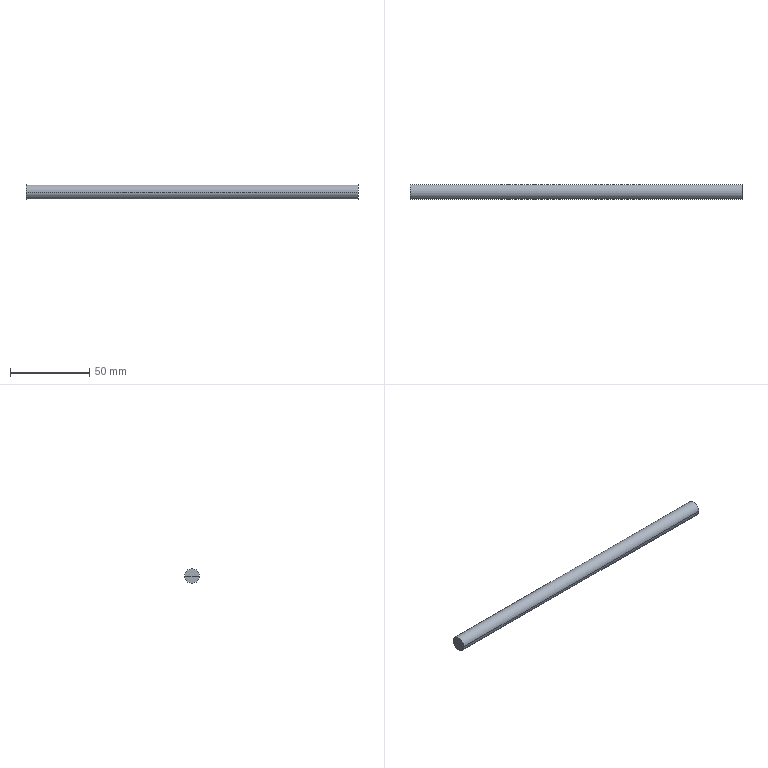Part | STEP file | BREP_8 | 1 solid | 6 faces | box 210 x 9.4 x 9.4 mm | volume 14574 mm3 | plane 4 | cylinder 2 | commonest cylinder face diameters 9.4 x2
STEP:
#1=CARTESIAN_POINT('',(0.,0.,0.));
#2=DIRECTION('',(0.,0.,1.));
#3=DIRECTION('',(1.,0.,0.));
#4=AXIS2_PLACEMENT_3D('',#1,#2,#3);
#5=CARTESIAN_POINT('',(-105.,0.,0.));
#6=VERTEX_POINT('',#5);
#7=CARTESIAN_POINT('',(-105.,-4.7,0.));
#8=VERTEX_POINT('',#7);
#9=CARTESIAN_POINT('',(-105.,0.,0.));
#10=DIRECTION('',(0.,-1.,0.));
#11=VECTOR('',#10,1.);
#12=LINE('',#9,#11);
#13=CARTESIAN_POINT('',(-105.,0.,-2.35));
#14=DIRECTION('',(1.,0.,0.));
#15=DIRECTION('',(0.,-1.,0.));
#16=AXIS2_PLACEMENT_3D('',#13,#14,#15);
#17=PLANE('',#16);
#18=CARTESIAN_POINT('',(0.,-2.35));
#19=DIRECTION('',(1.,0.));
#20=VECTOR('',#19,1.);
#21=LINE('',#18,#20);
#22=(GEOMETRIC_REPRESENTATION_CONTEXT(2)PARAMETRIC_REPRESENTATION_CONTEXT()REPRESENTATION_CONTEXT('',''));
#23=DEFINITIONAL_REPRESENTATION('',(#21),#22);
#24=PCURVE('',#17,#23);
#25=CARTESIAN_POINT('',(-105.,0.,2.35));
#26=DIRECTION('',(1.,0.,0.));
#27=DIRECTION('',(0.,1.,0.));
#28=AXIS2_PLACEMENT_3D('',#25,#26,#27);
#29=PLANE('',#28);
#30=CARTESIAN_POINT('',(0.,-2.35));
#31=DIRECTION('',(-1.,0.));
#32=VECTOR('',#31,1.);
#33=LINE('',#30,#32);
#34=(GEOMETRIC_REPRESENTATION_CONTEXT(2)PARAMETRIC_REPRESENTATION_CONTEXT()REPRESENTATION_CONTEXT('',''));
#35=DEFINITIONAL_REPRESENTATION('',(#33),#34);
#36=PCURVE('',#29,#35);
#37=SURFACE_CURVE('',#12,(#24,#36),.PCURVE_S1.);
#38=EDGE_CURVE('',#6,#8,#37,.T.);
#39=ORIENTED_EDGE('',*,*,#38,.T.);
#40=CARTESIAN_POINT('',(-105.,4.7,0.));
#41=VERTEX_POINT('',#40);
#42=CARTESIAN_POINT('',(-105.,0.,0.));
#43=DIRECTION('',(-1.,0.,0.));
#44=DIRECTION('',(0.,1.,0.));
#45=AXIS2_PLACEMENT_3D('',#42,#43,#44);
#46=CIRCLE('',#45,4.7);
#47=CARTESIAN_POINT('',(-4.7,-2.35));
#48=CARTESIAN_POINT('',(-4.7,5.791));
#49=CARTESIAN_POINT('',(2.35,1.72));
#50=CARTESIAN_POINT('',(9.4,-2.35));
#51=CARTESIAN_POINT('',(2.35,-6.42));
#52=CARTESIAN_POINT('',(-4.7,-10.491));
#53=CARTESIAN_POINT('',(-4.7,-2.35));
#54=(BOUNDED_CURVE()B_SPLINE_CURVE(2,(#47,#48,#49,#50,#51,#52,#53),.UNSPECIFIED.,.T.,.F.)B_SPLINE_CURVE_WITH_KNOTS((1,2,2,2,2,1),(-2.094,0.,2.094,4.189,6.283,8.378),.UNSPECIFIED.)CURVE()GEOMETRIC_REPRESENTATION_ITEM()RATIONAL_B_SPLINE_CURVE((1.,0.5,1.,0.5,1.,0.5,1.))REPRESENTATION_ITEM(''));
#55=(GEOMETRIC_REPRESENTATION_CONTEXT(2)PARAMETRIC_REPRESENTATION_CONTEXT()REPRESENTATION_CONTEXT('',''));
#56=DEFINITIONAL_REPRESENTATION('',(#54),#55);
#57=PCURVE('',#17,#56);
#58=CARTESIAN_POINT('',(0.,0.,0.));
#59=DIRECTION('',(-1.,0.,0.));
#60=DIRECTION('',(0.,1.,0.));
#61=AXIS2_PLACEMENT_3D('',#58,#59,#60);
#62=CYLINDRICAL_SURFACE('',#61,4.7);
#63=CARTESIAN_POINT('',(0.,105.));
#64=DIRECTION('',(1.,0.));
#65=VECTOR('',#64,1.);
#66=LINE('',#63,#65);
#67=(GEOMETRIC_REPRESENTATION_CONTEXT(2)PARAMETRIC_REPRESENTATION_CONTEXT()REPRESENTATION_CONTEXT('',''));
#68=DEFINITIONAL_REPRESENTATION('',(#66),#67);
#69=PCURVE('',#62,#68);
#70=SURFACE_CURVE('',#46,(#57,#69),.PCURVE_S1.);
#71=EDGE_CURVE('',#41,#8,#70,.T.);
#72=ORIENTED_EDGE('',*,*,#71,.F.);
#73=CARTESIAN_POINT('',(-105.,0.,0.));
#74=DIRECTION('',(0.,1.,0.));
#75=VECTOR('',#74,1.);
#76=LINE('',#73,#75);
#77=CARTESIAN_POINT('',(0.,-2.35));
#78=DIRECTION('',(-1.,0.));
#79=VECTOR('',#78,1.);
#80=LINE('',#77,#79);
#81=(GEOMETRIC_REPRESENTATION_CONTEXT(2)PARAMETRIC_REPRESENTATION_CONTEXT()REPRESENTATION_CONTEXT('',''));
#82=DEFINITIONAL_REPRESENTATION('',(#80),#81);
#83=PCURVE('',#17,#82);
#84=CARTESIAN_POINT('',(0.,-2.35));
#85=DIRECTION('',(1.,0.));
#86=VECTOR('',#85,1.);
#87=LINE('',#84,#86);
#88=(GEOMETRIC_REPRESENTATION_CONTEXT(2)PARAMETRIC_REPRESENTATION_CONTEXT()REPRESENTATION_CONTEXT('',''));
#89=DEFINITIONAL_REPRESENTATION('',(#87),#88);
#90=PCURVE('',#29,#89);
#91=SURFACE_CURVE('',#76,(#83,#90),.PCURVE_S1.);
#92=EDGE_CURVE('',#6,#41,#91,.T.);
#93=ORIENTED_EDGE('',*,*,#92,.F.);
#94=EDGE_LOOP('',(#39,#72,#93));
#95=FACE_BOUND('',#94,.F.);
#96=ADVANCED_FACE('',(#95),#17,.F.);
#97=CARTESIAN_POINT('',(-105.,0.,0.));
#98=DIRECTION('',(-1.,0.,0.));
#99=DIRECTION('',(0.,-1.,0.));
#100=AXIS2_PLACEMENT_3D('',#97,#98,#99);
#101=CIRCLE('',#100,4.7);
#102=CARTESIAN_POINT('',(-4.7,-2.35));
#103=CARTESIAN_POINT('',(-4.7,5.791));
#104=CARTESIAN_POINT('',(2.35,1.72));
#105=CARTESIAN_POINT('',(9.4,-2.35));
#106=CARTESIAN_POINT('',(2.35,-6.42));
#107=CARTESIAN_POINT('',(-4.7,-10.491));
#108=CARTESIAN_POINT('',(-4.7,-2.35));
#109=(BOUNDED_CURVE()B_SPLINE_CURVE(2,(#102,#103,#104,#105,#106,#107,#108),.UNSPECIFIED.,.T.,.F.)B_SPLINE_CURVE_WITH_KNOTS((1,2,2,2,2,1),(-2.094,0.,2.094,4.189,6.283,8.378),.UNSPECIFIED.)CURVE()GEOMETRIC_REPRESENTATION_ITEM()RATIONAL_B_SPLINE_CURVE((1.,0.5,1.,0.5,1.,0.5,1.))REPRESENTATION_ITEM(''));
#110=(GEOMETRIC_REPRESENTATION_CONTEXT(2)PARAMETRIC_REPRESENTATION_CONTEXT()REPRESENTATION_CONTEXT('',''));
#111=DEFINITIONAL_REPRESENTATION('',(#109),#110);
#112=PCURVE('',#29,#111);
#113=CARTESIAN_POINT('',(0.,0.,0.));
#114=DIRECTION('',(-1.,0.,0.));
#115=DIRECTION('',(0.,-1.,0.));
#116=AXIS2_PLACEMENT_3D('',#113,#114,#115);
#117=CYLINDRICAL_SURFACE('',#116,4.7);
#118=CARTESIAN_POINT('',(0.,105.));
#119=DIRECTION('',(1.,0.));
#120=VECTOR('',#119,1.);
#121=LINE('',#118,#120);
#122=(GEOMETRIC_REPRESENTATION_CONTEXT(2)PARAMETRIC_REPRESENTATION_CONTEXT()REPRESENTATION_CONTEXT('',''));
#123=DEFINITIONAL_REPRESENTATION('',(#121),#122);
#124=PCURVE('',#117,#123);
#125=SURFACE_CURVE('',#101,(#112,#124),.PCURVE_S1.);
#126=EDGE_CURVE('',#8,#41,#125,.T.);
#127=ORIENTED_EDGE('',*,*,#126,.F.);
#128=ORIENTED_EDGE('',*,*,#38,.F.);
#129=ORIENTED_EDGE('',*,*,#92,.T.);
#130=EDGE_LOOP('',(#127,#128,#129));
#131=FACE_BOUND('',#130,.F.);
#132=ADVANCED_FACE('',(#131),#29,.F.);
#133=CARTESIAN_POINT('',(105.,4.7,0.));
#134=VERTEX_POINT('',#133);
#135=CARTESIAN_POINT('',(-105.,4.7,0.));
#136=DIRECTION('',(1.,0.,0.));
#137=VECTOR('',#136,1.);
#138=LINE('',#135,#137);
#139=CARTESIAN_POINT('',(3.142,105.));
#140=DIRECTION('',(0.,-1.));
#141=VECTOR('',#140,1.);
#142=LINE('',#139,#141);
#143=(GEOMETRIC_REPRESENTATION_CONTEXT(2)PARAMETRIC_REPRESENTATION_CONTEXT()REPRESENTATION_CONTEXT('',''));
#144=DEFINITIONAL_REPRESENTATION('',(#142),#143);
#145=PCURVE('',#117,#144);
#146=CARTESIAN_POINT('',(0.,105.));
#147=DIRECTION('',(0.,-1.));
#148=VECTOR('',#147,1.);
#149=LINE('',#146,#148);
#150=(GEOMETRIC_REPRESENTATION_CONTEXT(2)PARAMETRIC_REPRESENTATION_CONTEXT()REPRESENTATION_CONTEXT('',''));
#151=DEFINITIONAL_REPRESENTATION('',(#149),#150);
#152=PCURVE('',#62,#151);
#153=SURFACE_CURVE('',#138,(#145,#152),.PCURVE_S1.);
#154=EDGE_CURVE('',#41,#134,#153,.T.);
#155=ORIENTED_EDGE('',*,*,#154,.F.);
#156=ORIENTED_EDGE('',*,*,#126,.F.);
#157=CARTESIAN_POINT('',(105.,-4.7,0.));
#158=VERTEX_POINT('',#157);
#159=CARTESIAN_POINT('',(-105.,-4.7,0.));
#160=DIRECTION('',(1.,0.,0.));
#161=VECTOR('',#160,1.);
#162=LINE('',#159,#161);
#163=CARTESIAN_POINT('',(0.,105.));
#164=DIRECTION('',(0.,-1.));
#165=VECTOR('',#164,1.);
#166=LINE('',#163,#165);
#167=(GEOMETRIC_REPRESENTATION_CONTEXT(2)PARAMETRIC_REPRESENTATION_CONTEXT()REPRESENTATION_CONTEXT('',''));
#168=DEFINITIONAL_REPRESENTATION('',(#166),#167);
#169=PCURVE('',#117,#168);
#170=CARTESIAN_POINT('',(3.142,105.));
#171=DIRECTION('',(0.,-1.));
#172=VECTOR('',#171,1.);
#173=LINE('',#170,#172);
#174=(GEOMETRIC_REPRESENTATION_CONTEXT(2)PARAMETRIC_REPRESENTATION_CONTEXT()REPRESENTATION_CONTEXT('',''));
#175=DEFINITIONAL_REPRESENTATION('',(#173),#174);
#176=PCURVE('',#62,#175);
#177=SURFACE_CURVE('',#162,(#169,#176),.PCURVE_S1.);
#178=EDGE_CURVE('',#8,#158,#177,.T.);
#179=ORIENTED_EDGE('',*,*,#178,.T.);
#180=CARTESIAN_POINT('',(105.,0.,0.));
#181=DIRECTION('',(1.,0.,0.));
#182=DIRECTION('',(0.,1.,0.));
#183=AXIS2_PLACEMENT_3D('',#180,#181,#182);
#184=CIRCLE('',#183,4.7);
#185=CARTESIAN_POINT('',(3.142,-105.));
#186=DIRECTION('',(-1.,0.));
#187=VECTOR('',#186,1.);
#188=LINE('',#185,#187);
#189=(GEOMETRIC_REPRESENTATION_CONTEXT(2)PARAMETRIC_REPRESENTATION_CONTEXT()REPRESENTATION_CONTEXT('',''));
#190=DEFINITIONAL_REPRESENTATION('',(#188),#189);
#191=PCURVE('',#117,#190);
#192=CARTESIAN_POINT('',(105.,0.,2.35));
#193=DIRECTION('',(1.,0.,0.));
#194=DIRECTION('',(0.,1.,0.));
#195=AXIS2_PLACEMENT_3D('',#192,#193,#194);
#196=PLANE('',#195);
#197=CARTESIAN_POINT('',(0.,-2.35));
#198=DIRECTION('',(1.,0.));
#199=AXIS2_PLACEMENT_2D('',#197,#198);
#200=CIRCLE('',#199,4.7);
#201=(GEOMETRIC_REPRESENTATION_CONTEXT(2)PARAMETRIC_REPRESENTATION_CONTEXT()REPRESENTATION_CONTEXT('',''));
#202=DEFINITIONAL_REPRESENTATION('',(#200),#201);
#203=PCURVE('',#196,#202);
#204=SURFACE_CURVE('',#184,(#191,#203),.PCURVE_S1.);
#205=EDGE_CURVE('',#134,#158,#204,.T.);
#206=ORIENTED_EDGE('',*,*,#205,.F.);
#207=EDGE_LOOP('',(#155,#156,#179,#206));
#208=FACE_BOUND('',#207,.T.);
#209=ADVANCED_FACE('',(#208),#117,.T.);
#210=CARTESIAN_POINT('',(105.,0.,0.));
#211=VERTEX_POINT('',#210);
#212=CARTESIAN_POINT('',(105.,4.7,0.));
#213=DIRECTION('',(0.,-1.,0.));
#214=VECTOR('',#213,1.);
#215=LINE('',#212,#214);
#216=CARTESIAN_POINT('',(4.7,-2.35));
#217=DIRECTION('',(-1.,0.));
#218=VECTOR('',#217,1.);
#219=LINE('',#216,#218);
#220=(GEOMETRIC_REPRESENTATION_CONTEXT(2)PARAMETRIC_REPRESENTATION_CONTEXT()REPRESENTATION_CONTEXT('',''));
#221=DEFINITIONAL_REPRESENTATION('',(#219),#220);
#222=PCURVE('',#196,#221);
#223=CARTESIAN_POINT('',(105.,0.,-2.35));
#224=DIRECTION('',(1.,0.,0.));
#225=DIRECTION('',(0.,-1.,0.));
#226=AXIS2_PLACEMENT_3D('',#223,#224,#225);
#227=PLANE('',#226);
#228=CARTESIAN_POINT('',(-4.7,-2.35));
#229=DIRECTION('',(1.,0.));
#230=VECTOR('',#229,1.);
#231=LINE('',#228,#230);
#232=(GEOMETRIC_REPRESENTATION_CONTEXT(2)PARAMETRIC_REPRESENTATION_CONTEXT()REPRESENTATION_CONTEXT('',''));
#233=DEFINITIONAL_REPRESENTATION('',(#231),#232);
#234=PCURVE('',#227,#233);
#235=SURFACE_CURVE('',#215,(#222,#234),.PCURVE_S1.);
#236=EDGE_CURVE('',#134,#211,#235,.T.);
#237=ORIENTED_EDGE('',*,*,#236,.T.);
#238=CARTESIAN_POINT('',(105.,-4.7,0.));
#239=DIRECTION('',(0.,1.,0.));
#240=VECTOR('',#239,1.);
#241=LINE('',#238,#240);
#242=CARTESIAN_POINT('',(-4.7,-2.35));
#243=DIRECTION('',(1.,0.));
#244=VECTOR('',#243,1.);
#245=LINE('',#242,#244);
#246=(GEOMETRIC_REPRESENTATION_CONTEXT(2)PARAMETRIC_REPRESENTATION_CONTEXT()REPRESENTATION_CONTEXT('',''));
#247=DEFINITIONAL_REPRESENTATION('',(#245),#246);
#248=PCURVE('',#196,#247);
#249=CARTESIAN_POINT('',(4.7,-2.35));
#250=DIRECTION('',(-1.,0.));
#251=VECTOR('',#250,1.);
#252=LINE('',#249,#251);
#253=(GEOMETRIC_REPRESENTATION_CONTEXT(2)PARAMETRIC_REPRESENTATION_CONTEXT()REPRESENTATION_CONTEXT('',''));
#254=DEFINITIONAL_REPRESENTATION('',(#252),#253);
#255=PCURVE('',#227,#254);
#256=SURFACE_CURVE('',#241,(#248,#255),.PCURVE_S1.);
#257=EDGE_CURVE('',#158,#211,#256,.T.);
#258=ORIENTED_EDGE('',*,*,#257,.F.);
#259=ORIENTED_EDGE('',*,*,#205,.F.);
#260=EDGE_LOOP('',(#237,#258,#259));
#261=FACE_BOUND('',#260,.F.);
#262=ADVANCED_FACE('',(#261),#196,.T.);
#263=ORIENTED_EDGE('',*,*,#257,.T.);
#264=ORIENTED_EDGE('',*,*,#236,.F.);
#265=CARTESIAN_POINT('',(105.,0.,0.));
#266=DIRECTION('',(1.,0.,0.));
#267=DIRECTION('',(0.,-1.,0.));
#268=AXIS2_PLACEMENT_3D('',#265,#266,#267);
#269=CIRCLE('',#268,4.7);
#270=CARTESIAN_POINT('',(0.,-2.35));
#271=DIRECTION('',(1.,0.));
#272=AXIS2_PLACEMENT_2D('',#270,#271);
#273=CIRCLE('',#272,4.7);
#274=(GEOMETRIC_REPRESENTATION_CONTEXT(2)PARAMETRIC_REPRESENTATION_CONTEXT()REPRESENTATION_CONTEXT('',''));
#275=DEFINITIONAL_REPRESENTATION('',(#273),#274);
#276=PCURVE('',#227,#275);
#277=CARTESIAN_POINT('',(3.142,-105.));
#278=DIRECTION('',(-1.,0.));
#279=VECTOR('',#278,1.);
#280=LINE('',#277,#279);
#281=(GEOMETRIC_REPRESENTATION_CONTEXT(2)PARAMETRIC_REPRESENTATION_CONTEXT()REPRESENTATION_CONTEXT('',''));
#282=DEFINITIONAL_REPRESENTATION('',(#280),#281);
#283=PCURVE('',#62,#282);
#284=SURFACE_CURVE('',#269,(#276,#283),.PCURVE_S1.);
#285=EDGE_CURVE('',#158,#134,#284,.T.);
#286=ORIENTED_EDGE('',*,*,#285,.F.);
#287=EDGE_LOOP('',(#263,#264,#286));
#288=FACE_BOUND('',#287,.F.);
#289=ADVANCED_FACE('',(#288),#227,.T.);
#290=ORIENTED_EDGE('',*,*,#71,.F.);
#291=ORIENTED_EDGE('',*,*,#154,.T.);
#292=ORIENTED_EDGE('',*,*,#285,.F.);
#293=ORIENTED_EDGE('',*,*,#178,.F.);
#294=EDGE_LOOP('',(#290,#291,#292,#293));
#295=FACE_BOUND('',#294,.T.);
#296=ADVANCED_FACE('',(#295),#62,.T.);
#297=CLOSED_SHELL('',(#96,#132,#209,#262,#289,#296));
#298=MANIFOLD_SOLID_BREP('',#297);
#299=(LENGTH_UNIT()NAMED_UNIT(*)SI_UNIT(.MILLI.,.METRE.));
#300=UNCERTAINTY_MEASURE_WITH_UNIT(LENGTH_MEASURE(0.0000001),#299,'','');
#301=(NAMED_UNIT(*)PLANE_ANGLE_UNIT()SI_UNIT($,.RADIAN.));
#302=(NAMED_UNIT(*)SI_UNIT($,.STERADIAN.)SOLID_ANGLE_UNIT());
#303=(GEOMETRIC_REPRESENTATION_CONTEXT(3)GLOBAL_UNCERTAINTY_ASSIGNED_CONTEXT((#300))GLOBAL_UNIT_ASSIGNED_CONTEXT((#299,#301,#302))REPRESENTATION_CONTEXT('',''));
#304=ADVANCED_BREP_SHAPE_REPRESENTATION('',(#4,#298),#303);